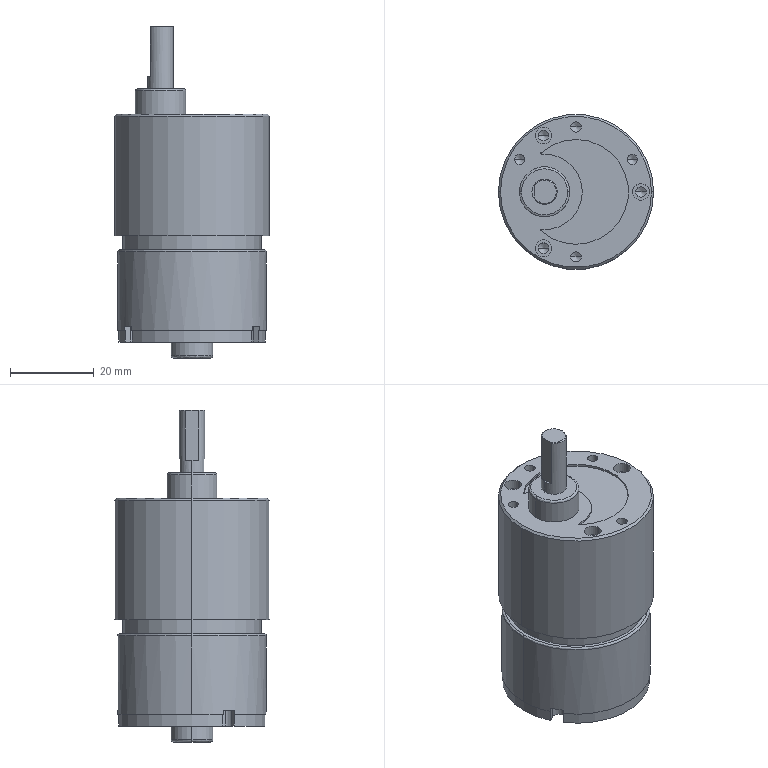Part | SolidWorks | features BaseBody 1 | 1 solid | 94 faces | box 37 x 37 x 79.2 mm | volume 56499 mm3 | cylinder 46 | plane 25 | cone 17 | spline 6 | commonest cylinder face diameters 2.459 x8 2.5 x6 4 x6 0.4 x4 3.243 x4 35 x4